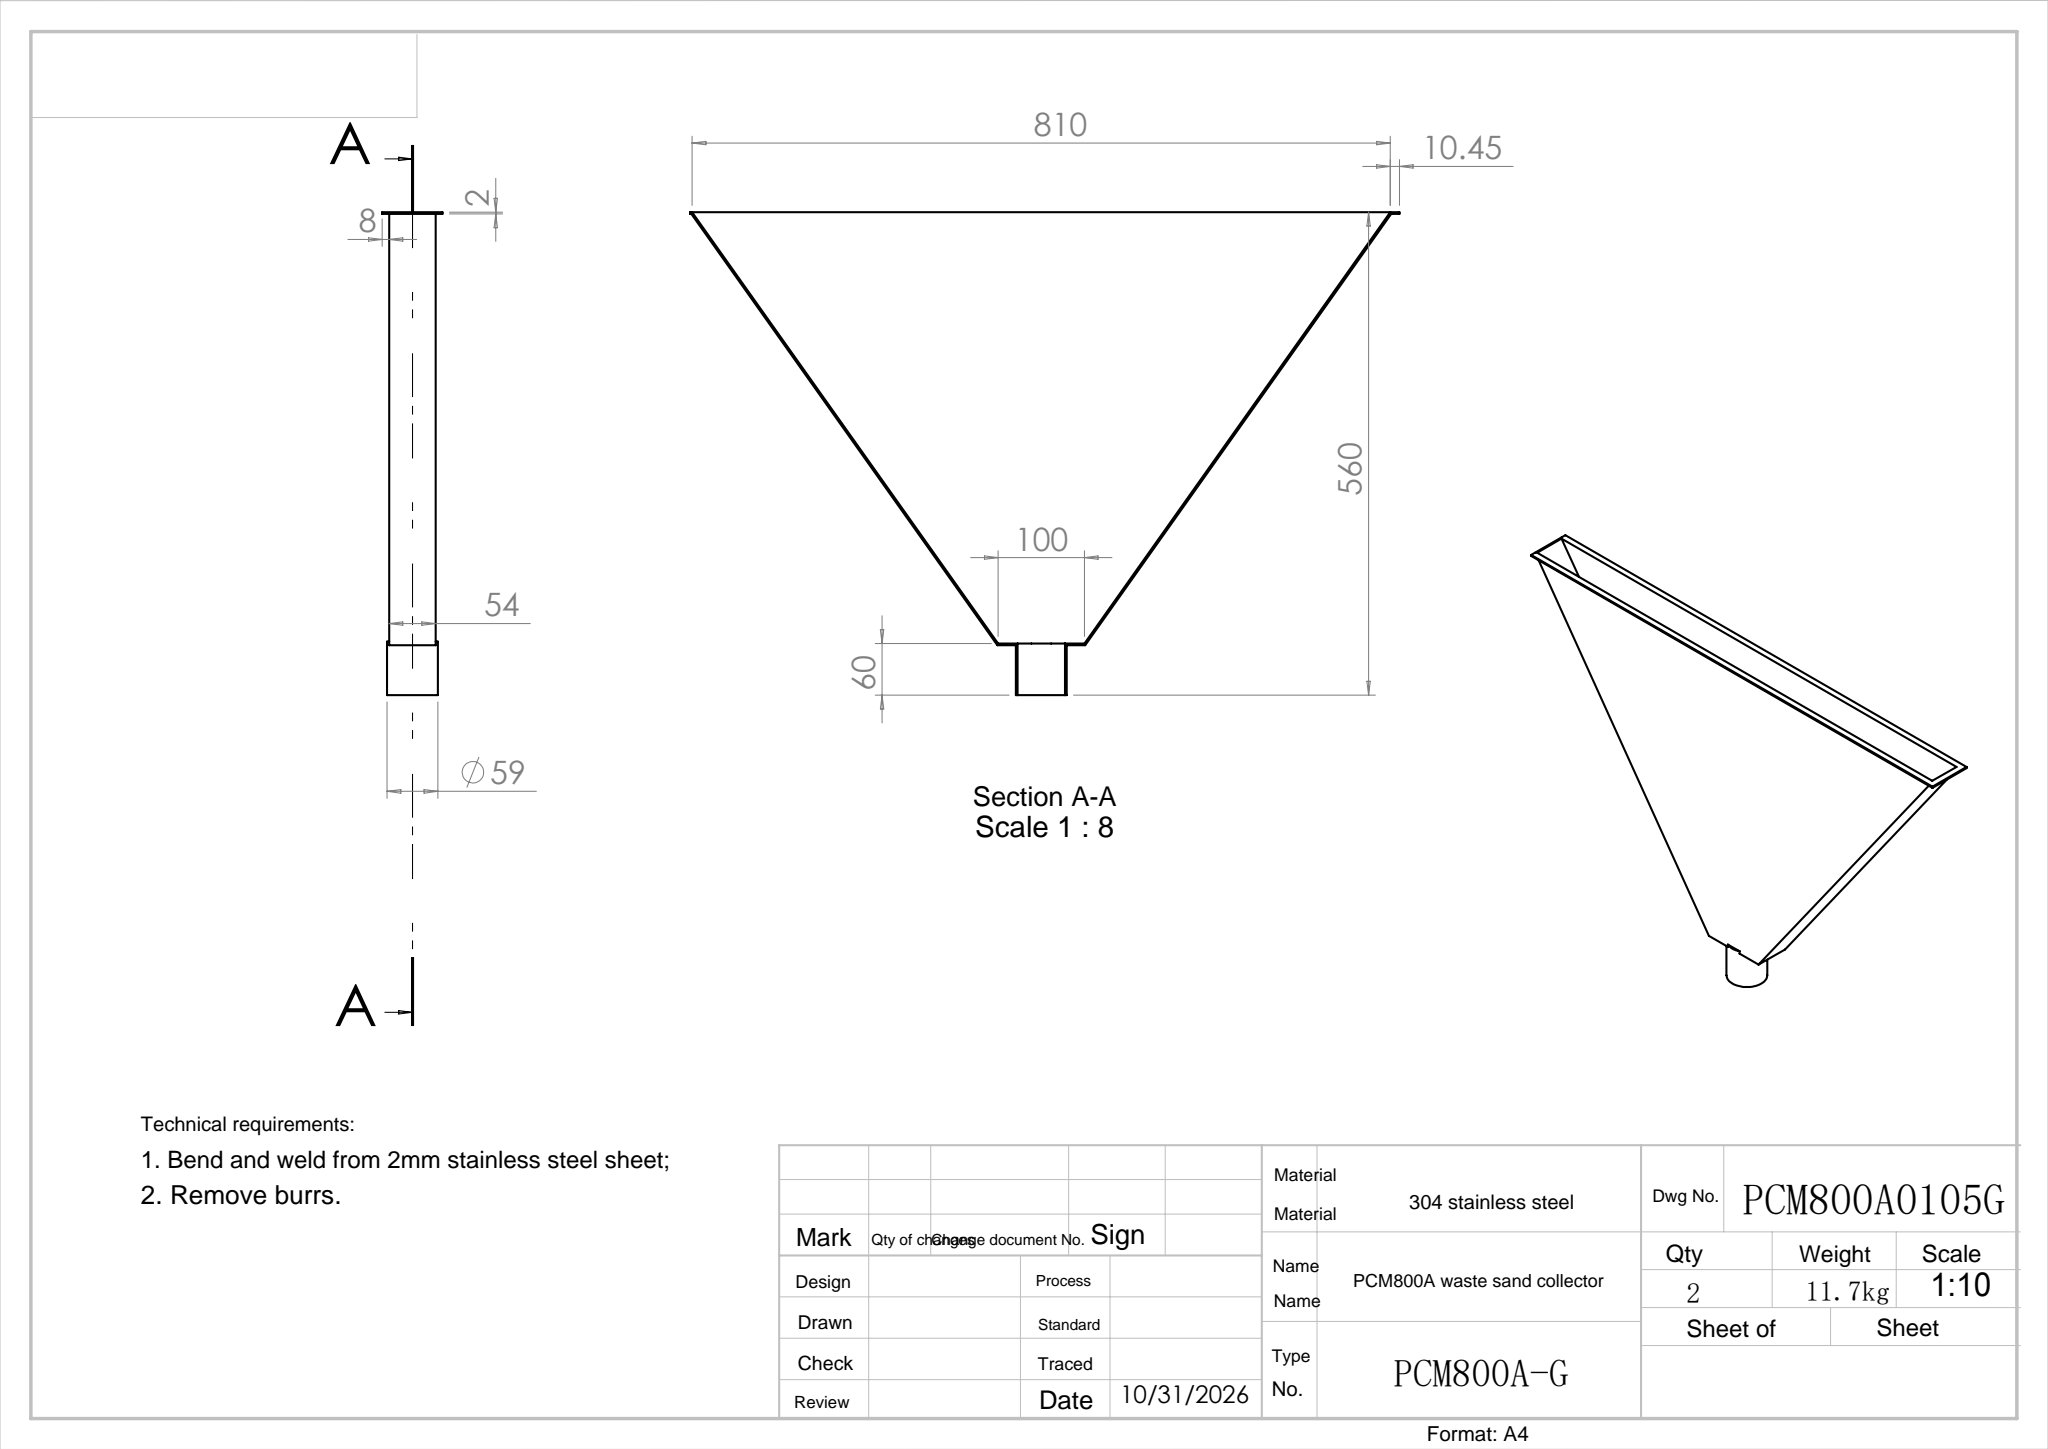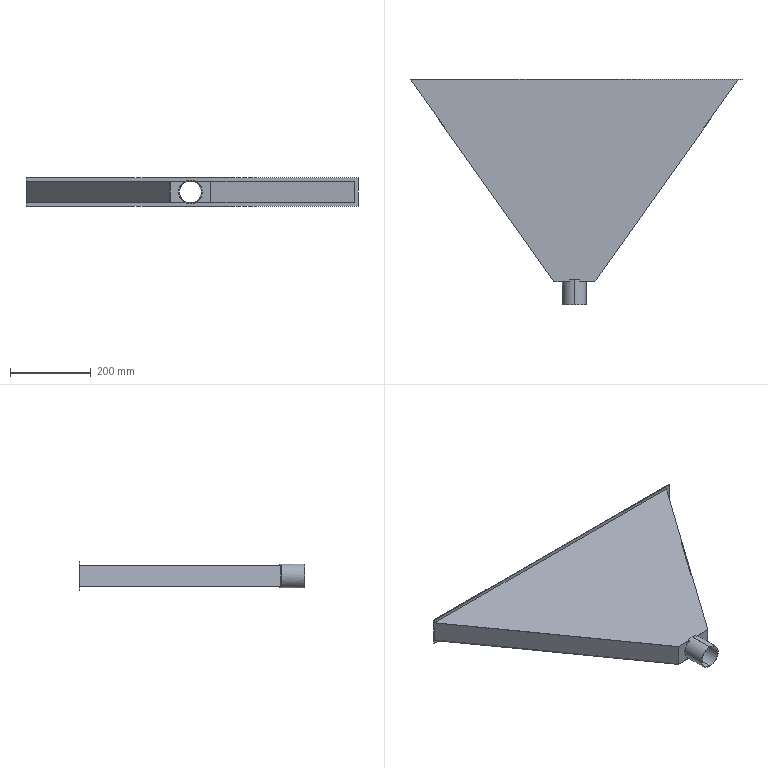Part | SolidWorks | features ICE 2, Extrusion 1, Shell 1 | 1 solid | 30 faces | box 822.906 x 560 x 70 mm | volume 1097243 mm3 | plane 26 | cylinder 4 | commonest cylinder face diameters 55 x2 59 x2
STEP:
#1=CARTESIAN_POINT('',(561.486,-560.,52.5));
#2=VERTEX_POINT('',#1);
#3=CARTESIAN_POINT('',(561.486,-560.,-2.5));
#4=VERTEX_POINT('',#3);
#5=CARTESIAN_POINT('',(561.486,-560.,25.));
#6=DIRECTION('',(0.,-1.,0.));
#7=DIRECTION('',(0.,0.,-1.));
#8=AXIS2_PLACEMENT_3D('',#5,#6,#7);
#9=CIRCLE('',#8,27.5);
#10=EDGE_CURVE('',#2,#4,#9,.T.);
#11=ORIENTED_EDGE('',*,*,#10,.T.);
#12=CARTESIAN_POINT('',(561.486,-500.,-2.5));
#13=VERTEX_POINT('',#12);
#14=CARTESIAN_POINT('',(561.486,-560.,-2.5));
#15=DIRECTION('',(0.,1.,0.));
#16=VECTOR('',#15,1000.);
#17=LINE('',#14,#16);
#18=EDGE_CURVE('',#4,#13,#17,.T.);
#19=ORIENTED_EDGE('',*,*,#18,.T.);
#20=CARTESIAN_POINT('',(550.03,-500.,0.));
#21=VERTEX_POINT('',#20);
#22=CARTESIAN_POINT('',(561.486,-500.,25.));
#23=DIRECTION('',(0.,-1.,0.));
#24=DIRECTION('',(0.,0.,-1.));
#25=AXIS2_PLACEMENT_3D('',#22,#23,#24);
#26=CIRCLE('',#25,27.5);
#27=EDGE_CURVE('',#21,#13,#26,.T.);
#28=ORIENTED_EDGE('',*,*,#27,.F.);
#29=CARTESIAN_POINT('',(550.03,-500.,50.));
#30=VERTEX_POINT('',#29);
#31=CARTESIAN_POINT('',(561.486,-500.,25.));
#32=DIRECTION('',(0.,-1.,0.));
#33=DIRECTION('',(0.,0.,-1.));
#34=AXIS2_PLACEMENT_3D('',#31,#32,#33);
#35=CIRCLE('',#34,27.5);
#36=EDGE_CURVE('',#30,#21,#35,.T.);
#37=ORIENTED_EDGE('',*,*,#36,.F.);
#38=CARTESIAN_POINT('',(561.486,-500.,52.5));
#39=VERTEX_POINT('',#38);
#40=CARTESIAN_POINT('',(561.486,-500.,25.));
#41=DIRECTION('',(0.,-1.,0.));
#42=DIRECTION('',(0.,0.,-1.));
#43=AXIS2_PLACEMENT_3D('',#40,#41,#42);
#44=CIRCLE('',#43,27.5);
#45=EDGE_CURVE('',#39,#30,#44,.T.);
#46=ORIENTED_EDGE('',*,*,#45,.F.);
#47=CARTESIAN_POINT('',(561.486,-560.,52.5));
#48=DIRECTION('',(0.,1.,0.));
#49=VECTOR('',#48,1000.);
#50=LINE('',#47,#49);
#51=EDGE_CURVE('',#2,#39,#50,.T.);
#52=ORIENTED_EDGE('',*,*,#51,.F.);
#53=EDGE_LOOP('',(#11,#19,#28,#37,#46,#52));
#54=FACE_OUTER_BOUND('',#53,.T.);
#55=CARTESIAN_POINT('',(561.486,-560.,25.));
#56=DIRECTION('',(0.,1.,0.));
#57=DIRECTION('',(0.,0.,1.));
#58=AXIS2_PLACEMENT_3D('',#55,#56,#57);
#59=CYLINDRICAL_SURFACE('',#58,27.5);
#60=ADVANCED_FACE('',(#54),#59,.F.);
#61=CARTESIAN_POINT('',(561.486,-560.,-4.5));
#62=VERTEX_POINT('',#61);
#63=CARTESIAN_POINT('',(561.486,-560.,54.5));
#64=VERTEX_POINT('',#63);
#65=CARTESIAN_POINT('',(561.486,-560.,25.));
#66=DIRECTION('',(0.,-1.,0.));
#67=DIRECTION('',(0.,0.,-1.));
#68=AXIS2_PLACEMENT_3D('',#65,#66,#67);
#69=CIRCLE('',#68,29.5);
#70=EDGE_CURVE('',#62,#64,#69,.T.);
#71=ORIENTED_EDGE('',*,*,#70,.F.);
#72=CARTESIAN_POINT('',(561.486,-498.,-4.5));
#73=VERTEX_POINT('',#72);
#74=CARTESIAN_POINT('',(561.486,-560.,-4.5));
#75=DIRECTION('',(0.,1.,0.));
#76=VECTOR('',#75,1000.);
#77=LINE('',#74,#76);
#78=EDGE_CURVE('',#62,#73,#77,.T.);
#79=ORIENTED_EDGE('',*,*,#78,.T.);
#80=CARTESIAN_POINT('',(573.371,-498.,-2.));
#81=VERTEX_POINT('',#80);
#82=CARTESIAN_POINT('',(561.486,-498.,25.));
#83=DIRECTION('',(0.,-1.,0.));
#84=DIRECTION('',(0.,0.,-1.));
#85=AXIS2_PLACEMENT_3D('',#82,#83,#84);
#86=CIRCLE('',#85,29.5);
#87=EDGE_CURVE('',#73,#81,#86,.T.);
#88=ORIENTED_EDGE('',*,*,#87,.T.);
#89=CARTESIAN_POINT('',(573.371,-502.,-2.));
#90=VERTEX_POINT('',#89);
#91=CARTESIAN_POINT('',(573.371,-502.,-2.));
#92=DIRECTION('',(0.,1.,0.));
#93=VECTOR('',#92,1000.);
#94=LINE('',#91,#93);
#95=EDGE_CURVE('',#90,#81,#94,.T.);
#96=ORIENTED_EDGE('',*,*,#95,.F.);
#97=CARTESIAN_POINT('',(573.371,-502.,52.));
#98=VERTEX_POINT('',#97);
#99=CARTESIAN_POINT('',(561.486,-502.,25.));
#100=DIRECTION('',(0.,-1.,0.));
#101=DIRECTION('',(-1.,0.,0.));
#102=AXIS2_PLACEMENT_3D('',#99,#100,#101);
#103=CIRCLE('',#102,29.5);
#104=EDGE_CURVE('',#90,#98,#103,.T.);
#105=ORIENTED_EDGE('',*,*,#104,.T.);
#106=CARTESIAN_POINT('',(573.371,-498.,52.));
#107=VERTEX_POINT('',#106);
#108=CARTESIAN_POINT('',(573.371,-502.,52.));
#109=DIRECTION('',(0.,1.,0.));
#110=VECTOR('',#109,1000.);
#111=LINE('',#108,#110);
#112=EDGE_CURVE('',#98,#107,#111,.T.);
#113=ORIENTED_EDGE('',*,*,#112,.T.);
#114=CARTESIAN_POINT('',(561.486,-498.,54.5));
#115=VERTEX_POINT('',#114);
#116=CARTESIAN_POINT('',(561.486,-498.,25.));
#117=DIRECTION('',(0.,-1.,0.));
#118=DIRECTION('',(0.,0.,-1.));
#119=AXIS2_PLACEMENT_3D('',#116,#117,#118);
#120=CIRCLE('',#119,29.5);
#121=EDGE_CURVE('',#107,#115,#120,.T.);
#122=ORIENTED_EDGE('',*,*,#121,.T.);
#123=CARTESIAN_POINT('',(561.486,-560.,54.5));
#124=DIRECTION('',(0.,1.,0.));
#125=VECTOR('',#124,1000.);
#126=LINE('',#123,#125);
#127=EDGE_CURVE('',#64,#115,#126,.T.);
#128=ORIENTED_EDGE('',*,*,#127,.F.);
#129=EDGE_LOOP('',(#71,#79,#88,#96,#105,#113,#122,#128));
#130=FACE_OUTER_BOUND('',#129,.T.);
#131=CARTESIAN_POINT('',(561.486,-560.,25.));
#132=DIRECTION('',(0.,1.,0.));
#133=DIRECTION('',(0.,0.,1.));
#134=AXIS2_PLACEMENT_3D('',#131,#132,#133);
#135=CYLINDRICAL_SURFACE('',#134,29.5);
#136=ADVANCED_FACE('',(#130),#135,.T.);
#137=CARTESIAN_POINT('',(967.519,-2.,52.));
#138=VERTEX_POINT('',#137);
#139=CARTESIAN_POINT('',(967.519,-2.,-2.));
#140=VERTEX_POINT('',#139);
#141=CARTESIAN_POINT('',(967.519,-2.,50.));
#142=DIRECTION('',(0.,0.,-1.));
#143=VECTOR('',#142,1000.);
#144=LINE('',#141,#143);
#145=EDGE_CURVE('',#138,#140,#144,.T.);
#146=ORIENTED_EDGE('',*,*,#145,.F.);
#147=CARTESIAN_POINT('',(612.519,-502.,52.));
#148=VERTEX_POINT('',#147);
#149=CARTESIAN_POINT('',(613.117,-501.158,52.));
#150=DIRECTION('',(0.5789,0.8154,0.));
#151=VECTOR('',#150,1000.);
#152=LINE('',#149,#151);
#153=EDGE_CURVE('',#148,#138,#152,.T.);
#154=ORIENTED_EDGE('',*,*,#153,.F.);
#155=CARTESIAN_POINT('',(612.519,-502.,-2.));
#156=VERTEX_POINT('',#155);
#157=CARTESIAN_POINT('',(612.519,-502.,50.));
#158=DIRECTION('',(0.,0.,-1.));
#159=VECTOR('',#158,1000.);
#160=LINE('',#157,#159);
#161=EDGE_CURVE('',#148,#156,#160,.T.);
#162=ORIENTED_EDGE('',*,*,#161,.T.);
#163=CARTESIAN_POINT('',(613.117,-501.158,-2.));
#164=DIRECTION('',(0.5789,0.8154,0.));
#165=VECTOR('',#164,1000.);
#166=LINE('',#163,#165);
#167=EDGE_CURVE('',#156,#140,#166,.T.);
#168=ORIENTED_EDGE('',*,*,#167,.T.);
#169=EDGE_LOOP('',(#146,#154,#162,#168));
#170=FACE_OUTER_BOUND('',#169,.T.);
#171=CARTESIAN_POINT('',(968.117,-1.158,50.));
#172=DIRECTION('',(-0.8154,0.5789,0.));
#173=DIRECTION('',(-0.5789,-0.8154,0.));
#174=AXIS2_PLACEMENT_3D('',#171,#172,#173);
#175=PLANE('',#174);
#176=ADVANCED_FACE('',(#170),#175,.F.);
#177=CARTESIAN_POINT('',(155.453,-2.,52.));
#178=VERTEX_POINT('',#177);
#179=CARTESIAN_POINT('',(611.486,-2.,52.));
#180=DIRECTION('',(1.,0.,0.));
#181=VECTOR('',#180,1000.);
#182=LINE('',#179,#181);
#183=EDGE_CURVE('',#178,#138,#182,.T.);
#184=ORIENTED_EDGE('',*,*,#183,.F.);
#185=CARTESIAN_POINT('',(510.453,-502.,52.));
#186=VERTEX_POINT('',#185);
#187=CARTESIAN_POINT('',(543.371,-548.362,52.));
#188=DIRECTION('',(0.5789,-0.8154,0.));
#189=VECTOR('',#188,1000.);
#190=LINE('',#187,#189);
#191=EDGE_CURVE('',#178,#186,#190,.T.);
#192=ORIENTED_EDGE('',*,*,#191,.T.);
#193=CARTESIAN_POINT('',(549.601,-502.,52.));
#194=VERTEX_POINT('',#193);
#195=CARTESIAN_POINT('',(611.486,-502.,52.));
#196=DIRECTION('',(1.,0.,0.));
#197=VECTOR('',#196,1000.);
#198=LINE('',#195,#197);
#199=EDGE_CURVE('',#186,#194,#198,.T.);
#200=ORIENTED_EDGE('',*,*,#199,.T.);
#201=CARTESIAN_POINT('',(549.601,-498.,52.));
#202=VERTEX_POINT('',#201);
#203=CARTESIAN_POINT('',(549.601,-502.,52.));
#204=DIRECTION('',(0.,1.,0.));
#205=VECTOR('',#204,1000.);
#206=LINE('',#203,#205);
#207=EDGE_CURVE('',#194,#202,#206,.T.);
#208=ORIENTED_EDGE('',*,*,#207,.T.);
#209=CARTESIAN_POINT('',(561.486,-498.,52.));
#210=DIRECTION('',(1.,0.,0.));
#211=VECTOR('',#210,1000.);
#212=LINE('',#209,#211);
#213=EDGE_CURVE('',#202,#107,#212,.T.);
#214=ORIENTED_EDGE('',*,*,#213,.T.);
#215=ORIENTED_EDGE('',*,*,#112,.F.);
#216=CARTESIAN_POINT('',(611.486,-502.,52.));
#217=DIRECTION('',(1.,0.,0.));
#218=VECTOR('',#217,1000.);
#219=LINE('',#216,#218);
#220=EDGE_CURVE('',#98,#148,#219,.T.);
#221=ORIENTED_EDGE('',*,*,#220,.T.);
#222=ORIENTED_EDGE('',*,*,#153,.T.);
#223=EDGE_LOOP('',(#184,#192,#200,#208,#214,#215,#221,#222));
#224=FACE_OUTER_BOUND('',#223,.T.);
#225=CARTESIAN_POINT('',(611.486,-500.,52.));
#226=DIRECTION('',(0.,0.,-1.));
#227=DIRECTION('',(-1.,0.,0.));
#228=AXIS2_PLACEMENT_3D('',#225,#226,#227);
#229=PLANE('',#228);
#230=ADVANCED_FACE('',(#224),#229,.F.);
#231=CARTESIAN_POINT('',(155.453,-2.,-2.));
#232=VERTEX_POINT('',#231);
#233=CARTESIAN_POINT('',(510.453,-502.,-2.));
#234=VERTEX_POINT('',#233);
#235=CARTESIAN_POINT('',(543.371,-548.362,-2.));
#236=DIRECTION('',(0.5789,-0.8154,0.));
#237=VECTOR('',#236,1000.);
#238=LINE('',#235,#237);
#239=EDGE_CURVE('',#232,#234,#238,.T.);
#240=ORIENTED_EDGE('',*,*,#239,.F.);
#241=CARTESIAN_POINT('',(611.486,-2.,-2.));
#242=DIRECTION('',(1.,0.,0.));
#243=VECTOR('',#242,1000.);
#244=LINE('',#241,#243);
#245=EDGE_CURVE('',#232,#140,#244,.T.);
#246=ORIENTED_EDGE('',*,*,#245,.T.);
#247=ORIENTED_EDGE('',*,*,#167,.F.);
#248=CARTESIAN_POINT('',(611.486,-502.,-2.));
#249=DIRECTION('',(1.,0.,0.));
#250=VECTOR('',#249,1000.);
#251=LINE('',#248,#250);
#252=EDGE_CURVE('',#90,#156,#251,.T.);
#253=ORIENTED_EDGE('',*,*,#252,.F.);
#254=ORIENTED_EDGE('',*,*,#95,.T.);
#255=CARTESIAN_POINT('',(549.601,-498.,-2.));
#256=VERTEX_POINT('',#255);
#257=CARTESIAN_POINT('',(561.486,-498.,-2.));
#258=DIRECTION('',(1.,0.,0.));
#259=VECTOR('',#258,1000.);
#260=LINE('',#257,#259);
#261=EDGE_CURVE('',#256,#81,#260,.T.);
#262=ORIENTED_EDGE('',*,*,#261,.F.);
#263=CARTESIAN_POINT('',(549.601,-502.,-2.));
#264=VERTEX_POINT('',#263);
#265=CARTESIAN_POINT('',(549.601,-502.,-2.));
#266=DIRECTION('',(0.,1.,0.));
#267=VECTOR('',#266,1000.);
#268=LINE('',#265,#267);
#269=EDGE_CURVE('',#264,#256,#268,.T.);
#270=ORIENTED_EDGE('',*,*,#269,.F.);
#271=CARTESIAN_POINT('',(611.486,-502.,-2.));
#272=DIRECTION('',(1.,0.,0.));
#273=VECTOR('',#272,1000.);
#274=LINE('',#271,#273);
#275=EDGE_CURVE('',#234,#264,#274,.T.);
#276=ORIENTED_EDGE('',*,*,#275,.F.);
#277=EDGE_LOOP('',(#240,#246,#247,#253,#254,#262,#270,#276));
#278=FACE_OUTER_BOUND('',#277,.T.);
#279=CARTESIAN_POINT('',(611.486,-500.,-2.));
#280=DIRECTION('',(0.,0.,-1.));
#281=DIRECTION('',(-1.,0.,0.));
#282=AXIS2_PLACEMENT_3D('',#279,#280,#281);
#283=PLANE('',#282);
#284=ADVANCED_FACE('',(#278),#283,.T.);
#285=CARTESIAN_POINT('',(966.486,0.,50.));
#286=VERTEX_POINT('',#285);
#287=CARTESIAN_POINT('',(966.486,0.,0.));
#288=VERTEX_POINT('',#287);
#289=CARTESIAN_POINT('',(966.486,0.,50.));
#290=DIRECTION('',(0.,0.,-1.));
#291=VECTOR('',#290,1000.);
#292=LINE('',#289,#291);
#293=EDGE_CURVE('',#286,#288,#292,.T.);
#294=ORIENTED_EDGE('',*,*,#293,.F.);
#295=CARTESIAN_POINT('',(156.486,0.,50.));
#296=VERTEX_POINT('',#295);
#297=CARTESIAN_POINT('',(966.486,0.,50.));
#298=DIRECTION('',(-1.,0.,0.));
#299=VECTOR('',#298,1000.);
#300=LINE('',#297,#299);
#301=EDGE_CURVE('',#286,#296,#300,.T.);
#302=ORIENTED_EDGE('',*,*,#301,.T.);
#303=CARTESIAN_POINT('',(156.486,0.,0.));
#304=VERTEX_POINT('',#303);
#305=CARTESIAN_POINT('',(156.486,0.,50.));
#306=DIRECTION('',(0.,0.,-1.));
#307=VECTOR('',#306,1000.);
#308=LINE('',#305,#307);
#309=EDGE_CURVE('',#296,#304,#308,.T.);
#310=ORIENTED_EDGE('',*,*,#309,.T.);
#311=CARTESIAN_POINT('',(966.486,0.,0.));
#312=DIRECTION('',(-1.,0.,0.));
#313=VECTOR('',#312,1000.);
#314=LINE('',#311,#313);
#315=EDGE_CURVE('',#288,#304,#314,.T.);
#316=ORIENTED_EDGE('',*,*,#315,.F.);
#317=EDGE_LOOP('',(#294,#302,#310,#316));
#318=FACE_BOUND('',#317,.T.);
#319=CARTESIAN_POINT('',(154.033,0.,52.));
#320=VERTEX_POINT('',#319);
#321=CARTESIAN_POINT('',(154.033,0.,-2.));
#322=VERTEX_POINT('',#321);
#323=CARTESIAN_POINT('',(154.033,0.,50.));
#324=DIRECTION('',(0.,0.,-1.));
#325=VECTOR('',#324,1000.);
#326=LINE('',#323,#325);
#327=EDGE_CURVE('',#320,#322,#326,.T.);
#328=ORIENTED_EDGE('',*,*,#327,.F.);
#329=CARTESIAN_POINT('',(154.033,0.,60.));
#330=VERTEX_POINT('',#329);
#331=CARTESIAN_POINT('',(154.033,0.,52.));
#332=DIRECTION('',(0.,0.,1.));
#333=VECTOR('',#332,1000.);
#334=LINE('',#331,#333);
#335=EDGE_CURVE('',#320,#330,#334,.T.);
#336=ORIENTED_EDGE('',*,*,#335,.T.);
#337=CARTESIAN_POINT('',(976.939,0.,60.));
#338=VERTEX_POINT('',#337);
#339=CARTESIAN_POINT('',(976.939,0.,60.));
#340=DIRECTION('',(1.,0.,0.));
#341=VECTOR('',#340,1000.);
#342=LINE('',#339,#341);
#343=EDGE_CURVE('',#330,#338,#342,.T.);
#344=ORIENTED_EDGE('',*,*,#343,.T.);
#345=CARTESIAN_POINT('',(976.939,0.,-10.));
#346=VERTEX_POINT('',#345);
#347=CARTESIAN_POINT('',(976.939,0.,-10.));
#348=DIRECTION('',(0.,0.,-1.));
#349=VECTOR('',#348,1000.);
#350=LINE('',#347,#349);
#351=EDGE_CURVE('',#338,#346,#350,.T.);
#352=ORIENTED_EDGE('',*,*,#351,.T.);
#353=CARTESIAN_POINT('',(154.033,0.,-10.));
#354=VERTEX_POINT('',#353);
#355=CARTESIAN_POINT('',(154.033,0.,-10.));
#356=DIRECTION('',(-1.,0.,0.));
#357=VECTOR('',#356,1000.);
#358=LINE('',#355,#357);
#359=EDGE_CURVE('',#346,#354,#358,.T.);
#360=ORIENTED_EDGE('',*,*,#359,.T.);
#361=CARTESIAN_POINT('',(154.033,0.,-10.));
#362=DIRECTION('',(0.,0.,1.));
#363=VECTOR('',#362,1000.);
#364=LINE('',#361,#363);
#365=EDGE_CURVE('',#354,#322,#364,.T.);
#366=ORIENTED_EDGE('',*,*,#365,.T.);
#367=EDGE_LOOP('',(#328,#336,#344,#352,#360,#366));
#368=FACE_OUTER_BOUND('',#367,.T.);
#369=CARTESIAN_POINT('',(966.486,0.,50.));
#370=DIRECTION('',(0.,-1.,0.));
#371=DIRECTION('',(1.,0.,0.));
#372=AXIS2_PLACEMENT_3D('',#369,#370,#371);
#373=PLANE('',#372);
#374=ADVANCED_FACE('',(#318,#368),#373,.F.);
#375=ORIENTED_EDGE('',*,*,#104,.F.);
#376=ORIENTED_EDGE('',*,*,#252,.T.);
#377=ORIENTED_EDGE('',*,*,#161,.F.);
#378=ORIENTED_EDGE('',*,*,#220,.F.);
#379=EDGE_LOOP('',(#375,#376,#377,#378));
#380=FACE_OUTER_BOUND('',#379,.T.);
#381=CARTESIAN_POINT('',(511.486,-502.,50.));
#382=DIRECTION('',(0.,1.,0.));
#383=DIRECTION('',(-1.,0.,0.));
#384=AXIS2_PLACEMENT_3D('',#381,#382,#383);
#385=PLANE('',#384);
#386=ADVANCED_FACE('',(#380),#385,.F.);
#387=CARTESIAN_POINT('',(561.486,-502.,25.));
#388=DIRECTION('',(0.,-1.,0.));
#389=DIRECTION('',(-1.,0.,0.));
#390=AXIS2_PLACEMENT_3D('',#387,#388,#389);
#391=CIRCLE('',#390,29.5);
#392=EDGE_CURVE('',#194,#264,#391,.T.);
#393=ORIENTED_EDGE('',*,*,#392,.F.);
#394=ORIENTED_EDGE('',*,*,#199,.F.);
#395=CARTESIAN_POINT('',(510.453,-502.,50.));
#396=DIRECTION('',(0.,0.,-1.));
#397=VECTOR('',#396,1000.);
#398=LINE('',#395,#397);
#399=EDGE_CURVE('',#186,#234,#398,.T.);
#400=ORIENTED_EDGE('',*,*,#399,.T.);
#401=ORIENTED_EDGE('',*,*,#275,.T.);
#402=EDGE_LOOP('',(#393,#394,#400,#401));
#403=FACE_OUTER_BOUND('',#402,.T.);
#404=CARTESIAN_POINT('',(511.486,-502.,50.));
#405=DIRECTION('',(0.,1.,0.));
#406=DIRECTION('',(-1.,0.,0.));
#407=AXIS2_PLACEMENT_3D('',#404,#405,#406);
#408=PLANE('',#407);
#409=ADVANCED_FACE('',(#403),#408,.F.);
#410=CARTESIAN_POINT('',(543.371,-548.362,-2.));
#411=DIRECTION('',(0.5789,-0.8154,0.));
#412=VECTOR('',#411,1000.);
#413=LINE('',#410,#412);
#414=EDGE_CURVE('',#322,#232,#413,.T.);
#415=ORIENTED_EDGE('',*,*,#414,.T.);
#416=ORIENTED_EDGE('',*,*,#239,.T.);
#417=ORIENTED_EDGE('',*,*,#399,.F.);
#418=ORIENTED_EDGE('',*,*,#191,.F.);
#419=CARTESIAN_POINT('',(543.371,-548.362,52.));
#420=DIRECTION('',(0.5789,-0.8154,0.));
#421=VECTOR('',#420,1000.);
#422=LINE('',#419,#421);
#423=EDGE_CURVE('',#320,#178,#422,.T.);
#424=ORIENTED_EDGE('',*,*,#423,.F.);
#425=ORIENTED_EDGE('',*,*,#327,.T.);
#426=EDGE_LOOP('',(#415,#416,#417,#418,#424,#425));
#427=FACE_OUTER_BOUND('',#426,.T.);
#428=CARTESIAN_POINT('',(154.856,-1.158,50.));
#429=DIRECTION('',(0.8154,0.5789,0.));
#430=DIRECTION('',(-0.5789,0.8154,0.));
#431=AXIS2_PLACEMENT_3D('',#428,#429,#430);
#432=PLANE('',#431);
#433=ADVANCED_FACE('',(#427),#432,.F.);
#434=CARTESIAN_POINT('',(561.486,-498.,25.));
#435=DIRECTION('',(0.,-1.,0.));
#436=DIRECTION('',(0.,0.,-1.));
#437=AXIS2_PLACEMENT_3D('',#434,#435,#436);
#438=CIRCLE('',#437,29.5);
#439=EDGE_CURVE('',#256,#73,#438,.T.);
#440=ORIENTED_EDGE('',*,*,#439,.F.);
#441=ORIENTED_EDGE('',*,*,#261,.T.);
#442=ORIENTED_EDGE('',*,*,#87,.F.);
#443=EDGE_LOOP('',(#440,#441,#442));
#444=FACE_OUTER_BOUND('',#443,.T.);
#445=CARTESIAN_POINT('',(561.486,-498.,25.));
#446=DIRECTION('',(0.,-1.,0.));
#447=DIRECTION('',(0.,0.,-1.));
#448=AXIS2_PLACEMENT_3D('',#445,#446,#447);
#449=PLANE('',#448);
#450=ADVANCED_FACE('',(#444),#449,.F.);
#451=ORIENTED_EDGE('',*,*,#78,.F.);
#452=CARTESIAN_POINT('',(561.486,-560.,25.));
#453=DIRECTION('',(0.,-1.,0.));
#454=DIRECTION('',(0.,0.,-1.));
#455=AXIS2_PLACEMENT_3D('',#452,#453,#454);
#456=CIRCLE('',#455,29.5);
#457=EDGE_CURVE('',#64,#62,#456,.T.);
#458=ORIENTED_EDGE('',*,*,#457,.F.);
#459=ORIENTED_EDGE('',*,*,#127,.T.);
#460=CARTESIAN_POINT('',(561.486,-498.,25.));
#461=DIRECTION('',(0.,-1.,0.));
#462=DIRECTION('',(0.,0.,-1.));
#463=AXIS2_PLACEMENT_3D('',#460,#461,#462);
#464=CIRCLE('',#463,29.5);
#465=EDGE_CURVE('',#115,#202,#464,.T.);
#466=ORIENTED_EDGE('',*,*,#465,.T.);
#467=ORIENTED_EDGE('',*,*,#207,.F.);
#468=ORIENTED_EDGE('',*,*,#392,.T.);
#469=ORIENTED_EDGE('',*,*,#269,.T.);
#470=ORIENTED_EDGE('',*,*,#439,.T.);
#471=EDGE_LOOP('',(#451,#458,#459,#466,#467,#468,#469,#470));
#472=FACE_OUTER_BOUND('',#471,.T.);
#473=CARTESIAN_POINT('',(561.486,-560.,25.));
#474=DIRECTION('',(0.,1.,0.));
#475=DIRECTION('',(0.,0.,1.));
#476=AXIS2_PLACEMENT_3D('',#473,#474,#475);
#477=CYLINDRICAL_SURFACE('',#476,29.5);
#478=ADVANCED_FACE('',(#472),#477,.T.);
#479=ORIENTED_EDGE('',*,*,#10,.F.);
#480=CARTESIAN_POINT('',(561.486,-560.,25.));
#481=DIRECTION('',(0.,-1.,0.));
#482=DIRECTION('',(0.,0.,-1.));
#483=AXIS2_PLACEMENT_3D('',#480,#481,#482);
#484=CIRCLE('',#483,27.5);
#485=EDGE_CURVE('',#4,#2,#484,.T.);
#486=ORIENTED_EDGE('',*,*,#485,.F.);
#487=EDGE_LOOP('',(#479,#486));
#488=FACE_BOUND('',#487,.T.);
#489=ORIENTED_EDGE('',*,*,#457,.T.);
#490=ORIENTED_EDGE('',*,*,#70,.T.);
#491=EDGE_LOOP('',(#489,#490));
#492=FACE_OUTER_BOUND('',#491,.T.);
#493=CARTESIAN_POINT('',(561.486,-560.,25.));
#494=DIRECTION('',(0.,-1.,0.));
#495=DIRECTION('',(0.,0.,-1.));
#496=AXIS2_PLACEMENT_3D('',#493,#494,#495);
#497=PLANE('',#496);
#498=ADVANCED_FACE('',(#488,#492),#497,.T.);
#499=ORIENTED_EDGE('',*,*,#213,.F.);
#500=ORIENTED_EDGE('',*,*,#465,.F.);
#501=ORIENTED_EDGE('',*,*,#121,.F.);
#502=EDGE_LOOP('',(#499,#500,#501));
#503=FACE_OUTER_BOUND('',#502,.T.);
#504=CARTESIAN_POINT('',(561.486,-498.,25.));
#505=DIRECTION('',(0.,-1.,0.));
#506=DIRECTION('',(0.,0.,-1.));
#507=AXIS2_PLACEMENT_3D('',#504,#505,#506);
#508=PLANE('',#507);
#509=ADVANCED_FACE('',(#503),#508,.F.);
#510=CARTESIAN_POINT('',(572.943,-500.,0.));
#511=VERTEX_POINT('',#510);
#512=CARTESIAN_POINT('',(572.943,-500.,50.));
#513=VERTEX_POINT('',#512);
#514=CARTESIAN_POINT('',(561.486,-500.,25.));
#515=DIRECTION('',(0.,-1.,0.));
#516=DIRECTION('',(0.,0.,-1.));
#517=AXIS2_PLACEMENT_3D('',#514,#515,#516);
#518=CIRCLE('',#517,27.5);
#519=EDGE_CURVE('',#511,#513,#518,.T.);
#520=ORIENTED_EDGE('',*,*,#519,.T.);
#521=CARTESIAN_POINT('',(611.486,-500.,50.));
#522=VERTEX_POINT('',#521);
#523=CARTESIAN_POINT('',(511.486,-500.,50.));
#524=DIRECTION('',(1.,0.,0.));
#525=VECTOR('',#524,1000.);
#526=LINE('',#523,#525);
#527=EDGE_CURVE('',#513,#522,#526,.T.);
#528=ORIENTED_EDGE('',*,*,#527,.T.);
#529=CARTESIAN_POINT('',(611.486,-500.,0.));
#530=VERTEX_POINT('',#529);
#531=CARTESIAN_POINT('',(611.486,-500.,50.));
#532=DIRECTION('',(0.,0.,-1.));
#533=VECTOR('',#532,1000.);
#534=LINE('',#531,#533);
#535=EDGE_CURVE('',#522,#530,#534,.T.);
#536=ORIENTED_EDGE('',*,*,#535,.T.);
#537=CARTESIAN_POINT('',(511.486,-500.,0.));
#538=DIRECTION('',(1.,0.,0.));
#539=VECTOR('',#538,1000.);
#540=LINE('',#537,#539);
#541=EDGE_CURVE('',#511,#530,#540,.T.);
#542=ORIENTED_EDGE('',*,*,#541,.F.);
#543=EDGE_LOOP('',(#520,#528,#536,#542));
#544=FACE_OUTER_BOUND('',#543,.T.);
#545=CARTESIAN_POINT('',(511.486,-500.,50.));
#546=DIRECTION('',(0.,1.,0.));
#547=DIRECTION('',(-1.,0.,0.));
#548=AXIS2_PLACEMENT_3D('',#545,#546,#547);
#549=PLANE('',#548);
#550=ADVANCED_FACE('',(#544),#549,.T.);
#551=ORIENTED_EDGE('',*,*,#36,.T.);
#552=CARTESIAN_POINT('',(511.486,-500.,0.));
#553=VERTEX_POINT('',#552);
#554=CARTESIAN_POINT('',(511.486,-500.,0.));
#555=DIRECTION('',(1.,0.,0.));
#556=VECTOR('',#555,1000.);
#557=LINE('',#554,#556);
#558=EDGE_CURVE('',#553,#21,#557,.T.);
#559=ORIENTED_EDGE('',*,*,#558,.F.);
#560=CARTESIAN_POINT('',(511.486,-500.,50.));
#561=VERTEX_POINT('',#560);
#562=CARTESIAN_POINT('',(511.486,-500.,50.));
#563=DIRECTION('',(0.,0.,-1.));
#564=VECTOR('',#563,1000.);
#565=LINE('',#562,#564);
#566=EDGE_CURVE('',#561,#553,#565,.T.);
#567=ORIENTED_EDGE('',*,*,#566,.F.);
#568=CARTESIAN_POINT('',(511.486,-500.,50.));
#569=DIRECTION('',(1.,0.,0.));
#570=VECTOR('',#569,1000.);
#571=LINE('',#568,#570);
#572=EDGE_CURVE('',#561,#30,#571,.T.);
#573=ORIENTED_EDGE('',*,*,#572,.T.);
#574=EDGE_LOOP('',(#551,#559,#567,#573));
#575=FACE_OUTER_BOUND('',#574,.T.);
#576=CARTESIAN_POINT('',(511.486,-500.,50.));
#577=DIRECTION('',(0.,1.,0.));
#578=DIRECTION('',(-1.,0.,0.));
#579=AXIS2_PLACEMENT_3D('',#576,#577,#578);
#580=PLANE('',#579);
#581=ADVANCED_FACE('',(#575),#580,.T.);
#582=CARTESIAN_POINT('',(966.486,0.,0.));
#583=DIRECTION('',(0.5789,0.8154,0.));
#584=VECTOR('',#583,1000.);
#585=LINE('',#582,#584);
#586=EDGE_CURVE('',#530,#288,#585,.T.);
#587=ORIENTED_EDGE('',*,*,#586,.F.);
#588=ORIENTED_EDGE('',*,*,#535,.F.);
#589=CARTESIAN_POINT('',(966.486,0.,50.));
#590=DIRECTION('',(0.5789,0.8154,0.));
#591=VECTOR('',#590,1000.);
#592=LINE('',#589,#591);
#593=EDGE_CURVE('',#522,#286,#592,.T.);
#594=ORIENTED_EDGE('',*,*,#593,.T.);
#595=ORIENTED_EDGE('',*,*,#293,.T.);
#596=EDGE_LOOP('',(#587,#588,#594,#595));
#597=FACE_OUTER_BOUND('',#596,.T.);
#598=CARTESIAN_POINT('',(966.486,0.,50.));
#599=DIRECTION('',(-0.8154,0.5789,0.));
#600=DIRECTION('',(-0.5789,-0.8154,0.));
#601=AXIS2_PLACEMENT_3D('',#598,#599,#600);
#602=PLANE('',#601);
#603=ADVANCED_FACE('',(#597),#602,.T.);
#604=CARTESIAN_POINT('',(156.486,0.,0.));
#605=DIRECTION('',(0.5789,-0.8154,0.));
#606=VECTOR('',#605,1000.);
#607=LINE('',#604,#606);
#608=EDGE_CURVE('',#304,#553,#607,.T.);
#609=ORIENTED_EDGE('',*,*,#608,.F.);
#610=ORIENTED_EDGE('',*,*,#309,.F.);
#611=CARTESIAN_POINT('',(156.486,0.,50.));
#612=DIRECTION('',(0.5789,-0.8154,0.));
#613=VECTOR('',#612,1000.);
#614=LINE('',#611,#613);
#615=EDGE_CURVE('',#296,#561,#614,.T.);
#616=ORIENTED_EDGE('',*,*,#615,.T.);
#617=ORIENTED_EDGE('',*,*,#566,.T.);
#618=EDGE_LOOP('',(#609,#610,#616,#617));
#619=FACE_OUTER_BOUND('',#618,.T.);
#620=CARTESIAN_POINT('',(156.486,0.,50.));
#621=DIRECTION('',(0.8154,0.5789,0.));
#622=DIRECTION('',(-0.5789,0.8154,0.));
#623=AXIS2_PLACEMENT_3D('',#620,#621,#622);
#624=PLANE('',#623);
#625=ADVANCED_FACE('',(#619),#624,.T.);
#626=ORIENTED_EDGE('',*,*,#572,.F.);
#627=ORIENTED_EDGE('',*,*,#615,.F.);
#628=ORIENTED_EDGE('',*,*,#301,.F.);
#629=ORIENTED_EDGE('',*,*,#593,.F.);
#630=ORIENTED_EDGE('',*,*,#527,.F.);
#631=CARTESIAN_POINT('',(511.486,-500.,50.));
#632=DIRECTION('',(1.,0.,0.));
#633=VECTOR('',#632,1000.);
#634=LINE('',#631,#633);
#635=EDGE_CURVE('',#30,#513,#634,.T.);
#636=ORIENTED_EDGE('',*,*,#635,.F.);
#637=EDGE_LOOP('',(#626,#627,#628,#629,#630,#636));
#638=FACE_OUTER_BOUND('',#637,.T.);
#639=CARTESIAN_POINT('',(611.486,-500.,50.));
#640=DIRECTION('',(0.,0.,-1.));
#641=DIRECTION('',(-1.,0.,0.));
#642=AXIS2_PLACEMENT_3D('',#639,#640,#641);
#643=PLANE('',#642);
#644=ADVANCED_FACE('',(#638),#643,.T.);
#645=ORIENTED_EDGE('',*,*,#558,.T.);
#646=CARTESIAN_POINT('',(511.486,-500.,0.));
#647=DIRECTION('',(1.,0.,0.));
#648=VECTOR('',#647,1000.);
#649=LINE('',#646,#648);
#650=EDGE_CURVE('',#21,#511,#649,.T.);
#651=ORIENTED_EDGE('',*,*,#650,.T.);
#652=ORIENTED_EDGE('',*,*,#541,.T.);
#653=ORIENTED_EDGE('',*,*,#586,.T.);
#654=ORIENTED_EDGE('',*,*,#315,.T.);
#655=ORIENTED_EDGE('',*,*,#608,.T.);
#656=EDGE_LOOP('',(#645,#651,#652,#653,#654,#655));
#657=FACE_OUTER_BOUND('',#656,.T.);
#658=CARTESIAN_POINT('',(611.486,-500.,0.));
#659=DIRECTION('',(0.,0.,-1.));
#660=DIRECTION('',(-1.,0.,0.));
#661=AXIS2_PLACEMENT_3D('',#658,#659,#660);
#662=PLANE('',#661);
#663=ADVANCED_FACE('',(#657),#662,.F.);
#664=ORIENTED_EDGE('',*,*,#27,.T.);
#665=CARTESIAN_POINT('',(561.486,-500.,25.));
#666=DIRECTION('',(0.,-1.,0.));
#667=DIRECTION('',(0.,0.,-1.));
#668=AXIS2_PLACEMENT_3D('',#665,#666,#667);
#669=CIRCLE('',#668,27.5);
#670=EDGE_CURVE('',#13,#511,#669,.T.);
#671=ORIENTED_EDGE('',*,*,#670,.T.);
#672=ORIENTED_EDGE('',*,*,#650,.F.);
#673=EDGE_LOOP('',(#664,#671,#672));
#674=FACE_OUTER_BOUND('',#673,.T.);
#675=CARTESIAN_POINT('',(561.486,-500.,25.));
#676=DIRECTION('',(0.,-1.,0.));
#677=DIRECTION('',(0.,0.,-1.));
#678=AXIS2_PLACEMENT_3D('',#675,#676,#677);
#679=PLANE('',#678);
#680=ADVANCED_FACE('',(#674),#679,.T.);
#681=ORIENTED_EDGE('',*,*,#18,.F.);
#682=ORIENTED_EDGE('',*,*,#485,.T.);
#683=ORIENTED_EDGE('',*,*,#51,.T.);
#684=CARTESIAN_POINT('',(561.486,-500.,25.));
#685=DIRECTION('',(0.,-1.,0.));
#686=DIRECTION('',(0.,0.,-1.));
#687=AXIS2_PLACEMENT_3D('',#684,#685,#686);
#688=CIRCLE('',#687,27.5);
#689=EDGE_CURVE('',#513,#39,#688,.T.);
#690=ORIENTED_EDGE('',*,*,#689,.F.);
#691=ORIENTED_EDGE('',*,*,#519,.F.);
#692=ORIENTED_EDGE('',*,*,#670,.F.);
#693=EDGE_LOOP('',(#681,#682,#683,#690,#691,#692));
#694=FACE_OUTER_BOUND('',#693,.T.);
#695=CARTESIAN_POINT('',(561.486,-560.,25.));
#696=DIRECTION('',(0.,1.,0.));
#697=DIRECTION('',(0.,0.,1.));
#698=AXIS2_PLACEMENT_3D('',#695,#696,#697);
#699=CYLINDRICAL_SURFACE('',#698,27.5);
#700=ADVANCED_FACE('',(#694),#699,.F.);
#701=ORIENTED_EDGE('',*,*,#635,.T.);
#702=ORIENTED_EDGE('',*,*,#689,.T.);
#703=ORIENTED_EDGE('',*,*,#45,.T.);
#704=EDGE_LOOP('',(#701,#702,#703));
#705=FACE_OUTER_BOUND('',#704,.T.);
#706=CARTESIAN_POINT('',(561.486,-500.,25.));
#707=DIRECTION('',(0.,-1.,0.));
#708=DIRECTION('',(0.,0.,-1.));
#709=AXIS2_PLACEMENT_3D('',#706,#707,#708);
#710=PLANE('',#709);
#711=ADVANCED_FACE('',(#705),#710,.T.);
#712=ORIENTED_EDGE('',*,*,#414,.F.);
#713=CARTESIAN_POINT('',(154.033,-2.,-2.));
#714=VERTEX_POINT('',#713);
#715=CARTESIAN_POINT('',(154.033,-2.,-2.));
#716=DIRECTION('',(0.,1.,0.));
#717=VECTOR('',#716,1000.);
#718=LINE('',#715,#717);
#719=EDGE_CURVE('',#714,#322,#718,.T.);
#720=ORIENTED_EDGE('',*,*,#719,.F.);
#721=CARTESIAN_POINT('',(154.033,-2.,-2.));
#722=DIRECTION('',(1.,0.,0.));
#723=VECTOR('',#722,1000.);
#724=LINE('',#721,#723);
#725=EDGE_CURVE('',#714,#232,#724,.T.);
#726=ORIENTED_EDGE('',*,*,#725,.T.);
#727=EDGE_LOOP('',(#712,#720,#726));
#728=FACE_OUTER_BOUND('',#727,.T.);
#729=CARTESIAN_POINT('',(154.033,-2.,-2.));
#730=DIRECTION('',(0.,0.,1.));
#731=DIRECTION('',(1.,0.,0.));
#732=AXIS2_PLACEMENT_3D('',#729,#730,#731);
#733=PLANE('',#732);
#734=ADVANCED_FACE('',(#728),#733,.T.);
#735=ORIENTED_EDGE('',*,*,#423,.T.);
#736=CARTESIAN_POINT('',(154.033,-2.,52.));
#737=VERTEX_POINT('',#736);
#738=CARTESIAN_POINT('',(966.486,-2.,52.));
#739=DIRECTION('',(-1.,0.,0.));
#740=VECTOR('',#739,1000.);
#741=LINE('',#738,#740);
#742=EDGE_CURVE('',#178,#737,#741,.T.);
#743=ORIENTED_EDGE('',*,*,#742,.T.);
#744=CARTESIAN_POINT('',(154.033,-2.,52.));
#745=DIRECTION('',(0.,1.,0.));
#746=VECTOR('',#745,1000.);
#747=LINE('',#744,#746);
#748=EDGE_CURVE('',#737,#320,#747,.T.);
#749=ORIENTED_EDGE('',*,*,#748,.T.);
#750=EDGE_LOOP('',(#735,#743,#749));
#751=FACE_OUTER_BOUND('',#750,.T.);
#752=CARTESIAN_POINT('',(966.486,-2.,52.));
#753=DIRECTION('',(0.,0.,-1.));
#754=DIRECTION('',(-1.,0.,0.));
#755=AXIS2_PLACEMENT_3D('',#752,#753,#754);
#756=PLANE('',#755);
#757=ADVANCED_FACE('',(#751),#756,.T.);
#758=ORIENTED_EDGE('',*,*,#742,.F.);
#759=ORIENTED_EDGE('',*,*,#183,.T.);
#760=ORIENTED_EDGE('',*,*,#145,.T.);
#761=ORIENTED_EDGE('',*,*,#245,.F.);
#762=ORIENTED_EDGE('',*,*,#725,.F.);
#763=CARTESIAN_POINT('',(154.033,-2.,-10.));
#764=VERTEX_POINT('',#763);
#765=CARTESIAN_POINT('',(154.033,-2.,-10.));
#766=DIRECTION('',(0.,0.,1.));
#767=VECTOR('',#766,1000.);
#768=LINE('',#765,#767);
#769=EDGE_CURVE('',#764,#714,#768,.T.);
#770=ORIENTED_EDGE('',*,*,#769,.F.);
#771=CARTESIAN_POINT('',(976.939,-2.,-10.));
#772=VERTEX_POINT('',#771);
#773=CARTESIAN_POINT('',(154.033,-2.,-10.));
#774=DIRECTION('',(-1.,0.,0.));
#775=VECTOR('',#774,1000.);
#776=LINE('',#773,#775);
#777=EDGE_CURVE('',#772,#764,#776,.T.);
#778=ORIENTED_EDGE('',*,*,#777,.F.);
#779=CARTESIAN_POINT('',(976.939,-2.,60.));
#780=VERTEX_POINT('',#779);
#781=CARTESIAN_POINT('',(976.939,-2.,-10.));
#782=DIRECTION('',(0.,0.,-1.));
#783=VECTOR('',#782,1000.);
#784=LINE('',#781,#783);
#785=EDGE_CURVE('',#780,#772,#784,.T.);
#786=ORIENTED_EDGE('',*,*,#785,.F.);
#787=CARTESIAN_POINT('',(154.033,-2.,60.));
#788=VERTEX_POINT('',#787);
#789=CARTESIAN_POINT('',(976.939,-2.,60.));
#790=DIRECTION('',(1.,0.,0.));
#791=VECTOR('',#790,1000.);
#792=LINE('',#789,#791);
#793=EDGE_CURVE('',#788,#780,#792,.T.);
#794=ORIENTED_EDGE('',*,*,#793,.F.);
#795=CARTESIAN_POINT('',(154.033,-2.,52.));
#796=DIRECTION('',(0.,0.,1.));
#797=VECTOR('',#796,1000.);
#798=LINE('',#795,#797);
#799=EDGE_CURVE('',#737,#788,#798,.T.);
#800=ORIENTED_EDGE('',*,*,#799,.F.);
#801=EDGE_LOOP('',(#758,#759,#760,#761,#762,#770,#778,#786,#794,#800));
#802=FACE_OUTER_BOUND('',#801,.T.);
#803=CARTESIAN_POINT('',(966.486,-2.,-2.));
#804=DIRECTION('',(0.,1.,0.));
#805=DIRECTION('',(-1.,0.,0.));
#806=AXIS2_PLACEMENT_3D('',#803,#804,#805);
#807=PLANE('',#806);
#808=ADVANCED_FACE('',(#802),#807,.F.);
#809=ORIENTED_EDGE('',*,*,#365,.F.);
#810=CARTESIAN_POINT('',(154.033,-2.,-10.));
#811=DIRECTION('',(0.,1.,0.));
#812=VECTOR('',#811,1000.);
#813=LINE('',#810,#812);
#814=EDGE_CURVE('',#764,#354,#813,.T.);
#815=ORIENTED_EDGE('',*,*,#814,.F.);
#816=ORIENTED_EDGE('',*,*,#769,.T.);
#817=ORIENTED_EDGE('',*,*,#719,.T.);
#818=EDGE_LOOP('',(#809,#815,#816,#817));
#819=FACE_OUTER_BOUND('',#818,.T.);
#820=CARTESIAN_POINT('',(154.033,-2.,-10.));
#821=DIRECTION('',(-1.,0.,0.));
#822=DIRECTION('',(0.,0.,1.));
#823=AXIS2_PLACEMENT_3D('',#820,#821,#822);
#824=PLANE('',#823);
#825=ADVANCED_FACE('',(#819),#824,.T.);
#826=ORIENTED_EDGE('',*,*,#359,.F.);
#827=CARTESIAN_POINT('',(976.939,-2.,-10.));
#828=DIRECTION('',(0.,1.,0.));
#829=VECTOR('',#828,1000.);
#830=LINE('',#827,#829);
#831=EDGE_CURVE('',#772,#346,#830,.T.);
#832=ORIENTED_EDGE('',*,*,#831,.F.);
#833=ORIENTED_EDGE('',*,*,#777,.T.);
#834=ORIENTED_EDGE('',*,*,#814,.T.);
#835=EDGE_LOOP('',(#826,#832,#833,#834));
#836=FACE_OUTER_BOUND('',#835,.T.);
#837=CARTESIAN_POINT('',(154.033,-2.,-10.));
#838=DIRECTION('',(0.,0.,-1.));
#839=DIRECTION('',(-1.,0.,0.));
#840=AXIS2_PLACEMENT_3D('',#837,#838,#839);
#841=PLANE('',#840);
#842=ADVANCED_FACE('',(#836),#841,.T.);
#843=ORIENTED_EDGE('',*,*,#351,.F.);
#844=CARTESIAN_POINT('',(976.939,-2.,60.));
#845=DIRECTION('',(0.,1.,0.));
#846=VECTOR('',#845,1000.);
#847=LINE('',#844,#846);
#848=EDGE_CURVE('',#780,#338,#847,.T.);
#849=ORIENTED_EDGE('',*,*,#848,.F.);
#850=ORIENTED_EDGE('',*,*,#785,.T.);
#851=ORIENTED_EDGE('',*,*,#831,.T.);
#852=EDGE_LOOP('',(#843,#849,#850,#851));
#853=FACE_OUTER_BOUND('',#852,.T.);
#854=CARTESIAN_POINT('',(976.939,-2.,-10.));
#855=DIRECTION('',(1.,0.,0.));
#856=DIRECTION('',(0.,1.,0.));
#857=AXIS2_PLACEMENT_3D('',#854,#855,#856);
#858=PLANE('',#857);
#859=ADVANCED_FACE('',(#853),#858,.T.);
#860=ORIENTED_EDGE('',*,*,#343,.F.);
#861=CARTESIAN_POINT('',(154.033,-2.,60.));
#862=DIRECTION('',(0.,1.,0.));
#863=VECTOR('',#862,1000.);
#864=LINE('',#861,#863);
#865=EDGE_CURVE('',#788,#330,#864,.T.);
#866=ORIENTED_EDGE('',*,*,#865,.F.);
#867=ORIENTED_EDGE('',*,*,#793,.T.);
#868=ORIENTED_EDGE('',*,*,#848,.T.);
#869=EDGE_LOOP('',(#860,#866,#867,#868));
#870=FACE_OUTER_BOUND('',#869,.T.);
#871=CARTESIAN_POINT('',(976.939,-2.,60.));
#872=DIRECTION('',(0.,0.,1.));
#873=DIRECTION('',(1.,0.,0.));
#874=AXIS2_PLACEMENT_3D('',#871,#872,#873);
#875=PLANE('',#874);
#876=ADVANCED_FACE('',(#870),#875,.T.);
#877=ORIENTED_EDGE('',*,*,#335,.F.);
#878=ORIENTED_EDGE('',*,*,#748,.F.);
#879=ORIENTED_EDGE('',*,*,#799,.T.);
#880=ORIENTED_EDGE('',*,*,#865,.T.);
#881=EDGE_LOOP('',(#877,#878,#879,#880));
#882=FACE_OUTER_BOUND('',#881,.T.);
#883=CARTESIAN_POINT('',(154.033,-2.,52.));
#884=DIRECTION('',(-1.,0.,0.));
#885=DIRECTION('',(0.,0.,1.));
#886=AXIS2_PLACEMENT_3D('',#883,#884,#885);
#887=PLANE('',#886);
#888=ADVANCED_FACE('',(#882),#887,.T.);
#889=CLOSED_SHELL('',(#60,#136,#176,#230,#284,#374,#386,#409,#433,#450,#478,#498,#509,#550,#581,#603,#625,#644,#663,#680,#700,#711,#734,#757,#808,#825,#842,#859,#876,#888));
#890=MANIFOLD_SOLID_BREP('',#889);
#891=CARTESIAN_POINT('',(0.,0.,0.));
#892=DIRECTION('',(0.,0.,1.));
#893=DIRECTION('',(1.,0.,0.));
#894=AXIS2_PLACEMENT_3D('',#891,#892,#893);
#895=(LENGTH_UNIT()NAMED_UNIT(*)SI_UNIT(.MILLI.,.METRE.));
#896=UNCERTAINTY_MEASURE_WITH_UNIT(LENGTH_MEASURE(0.00001),#895,'','');
#897=(NAMED_UNIT(*)PLANE_ANGLE_UNIT()SI_UNIT($,.RADIAN.));
#898=(NAMED_UNIT(*)SI_UNIT($,.STERADIAN.)SOLID_ANGLE_UNIT());
#899=(GEOMETRIC_REPRESENTATION_CONTEXT(3)GLOBAL_UNCERTAINTY_ASSIGNED_CONTEXT((#896))GLOBAL_UNIT_ASSIGNED_CONTEXT((#895,#897,#898))REPRESENTATION_CONTEXT('',''));
#900=ADVANCED_BREP_SHAPE_REPRESENTATION('',(#890,#894),#899);